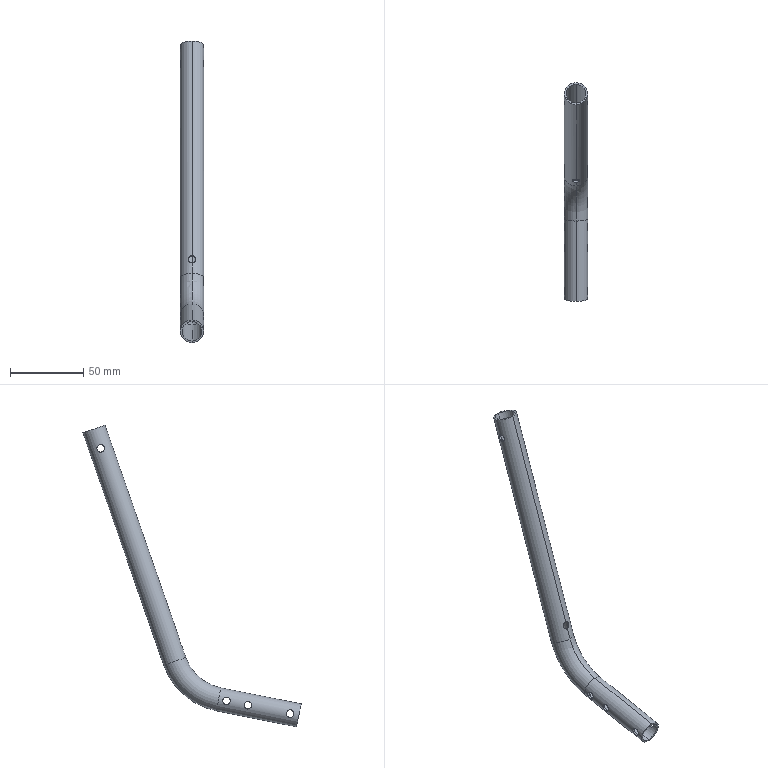Part | SolidWorks | features BaseBody 1 | 1 solid | 32 faces | box 16 x 149.335 x 206.465 mm | volume 14602 mm3 | cylinder 26 | torus 4 | plane 2 | commonest cylinder face diameters 5.2 x18 13.6 x4 16 x4